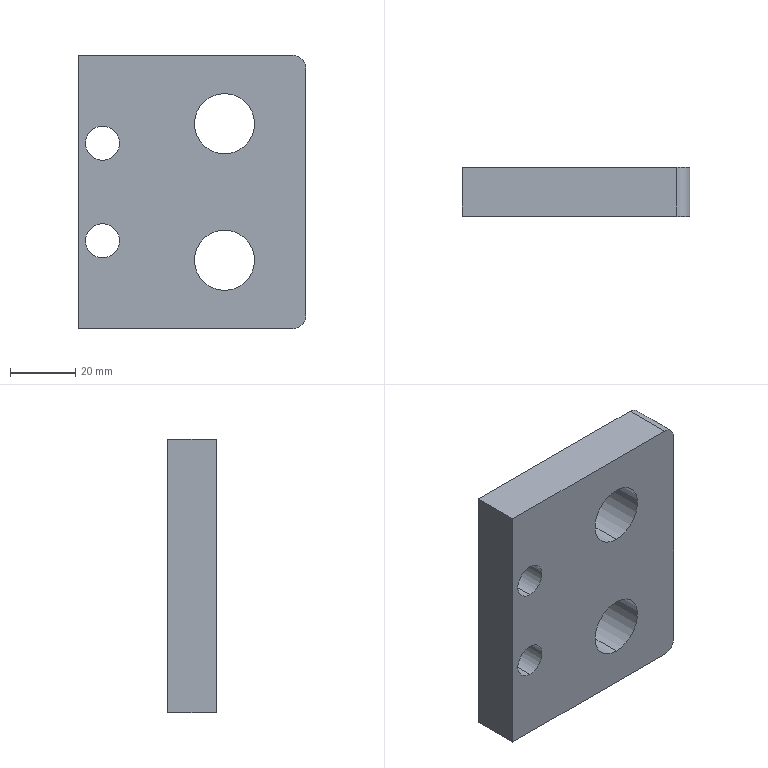Part | 1 solid | 16 faces | box 70 x 15 x 84 mm | volume 77435 mm3 | cylinder 10 | plane 6 | commonest cylinder face diameters 10.5 x4 18.5 x4 8 x2
STEP:
#1=CARTESIAN_POINT('',(10.,0.,-30.25));
#2=VERTEX_POINT('',#1);
#3=CARTESIAN_POINT('',(10.,0.,-11.75));
#4=VERTEX_POINT('',#3);
#5=CARTESIAN_POINT('',(10.,0.,-21.));
#6=DIRECTION('',(0.,1.,0.));
#7=DIRECTION('',(0.,0.,1.));
#8=AXIS2_PLACEMENT_3D('',#5,#6,#7);
#9=CIRCLE('',#8,9.25);
#10=EDGE_CURVE('',#2,#4,#9,.T.);
#11=ORIENTED_EDGE('',*,*,#10,.F.);
#12=CARTESIAN_POINT('',(10.,15.,-30.25));
#13=VERTEX_POINT('',#12);
#14=CARTESIAN_POINT('',(10.,15.,-30.25));
#15=DIRECTION('',(0.,1.,0.));
#16=VECTOR('',#15,1000.);
#17=LINE('',#14,#16);
#18=EDGE_CURVE('',#2,#13,#17,.T.);
#19=ORIENTED_EDGE('',*,*,#18,.T.);
#20=CARTESIAN_POINT('',(10.,15.,-11.75));
#21=VERTEX_POINT('',#20);
#22=CARTESIAN_POINT('',(10.,15.,-21.));
#23=DIRECTION('',(0.,1.,0.));
#24=DIRECTION('',(0.,0.,1.));
#25=AXIS2_PLACEMENT_3D('',#22,#23,#24);
#26=CIRCLE('',#25,9.25);
#27=EDGE_CURVE('',#13,#21,#26,.T.);
#28=ORIENTED_EDGE('',*,*,#27,.T.);
#29=CARTESIAN_POINT('',(10.,15.,-11.75));
#30=DIRECTION('',(0.,1.,0.));
#31=VECTOR('',#30,1000.);
#32=LINE('',#29,#31);
#33=EDGE_CURVE('',#4,#21,#32,.T.);
#34=ORIENTED_EDGE('',*,*,#33,.F.);
#35=EDGE_LOOP('',(#11,#19,#28,#34));
#36=FACE_OUTER_BOUND('',#35,.T.);
#37=CARTESIAN_POINT('',(10.,15.,-21.));
#38=DIRECTION('',(0.,1.,0.));
#39=DIRECTION('',(0.,0.,1.));
#40=AXIS2_PLACEMENT_3D('',#37,#38,#39);
#41=CYLINDRICAL_SURFACE('',#40,9.25);
#42=ADVANCED_FACE('',(#36),#41,.F.);
#43=CARTESIAN_POINT('',(10.,0.,11.75));
#44=VERTEX_POINT('',#43);
#45=CARTESIAN_POINT('',(10.,0.,30.25));
#46=VERTEX_POINT('',#45);
#47=CARTESIAN_POINT('',(10.,0.,21.));
#48=DIRECTION('',(0.,1.,0.));
#49=DIRECTION('',(0.,0.,1.));
#50=AXIS2_PLACEMENT_3D('',#47,#48,#49);
#51=CIRCLE('',#50,9.25);
#52=EDGE_CURVE('',#44,#46,#51,.T.);
#53=ORIENTED_EDGE('',*,*,#52,.F.);
#54=CARTESIAN_POINT('',(10.,15.,11.75));
#55=VERTEX_POINT('',#54);
#56=CARTESIAN_POINT('',(10.,15.,11.75));
#57=DIRECTION('',(0.,1.,0.));
#58=VECTOR('',#57,1000.);
#59=LINE('',#56,#58);
#60=EDGE_CURVE('',#44,#55,#59,.T.);
#61=ORIENTED_EDGE('',*,*,#60,.T.);
#62=CARTESIAN_POINT('',(10.,15.,30.25));
#63=VERTEX_POINT('',#62);
#64=CARTESIAN_POINT('',(10.,15.,21.));
#65=DIRECTION('',(0.,1.,0.));
#66=DIRECTION('',(0.,0.,1.));
#67=AXIS2_PLACEMENT_3D('',#64,#65,#66);
#68=CIRCLE('',#67,9.25);
#69=EDGE_CURVE('',#55,#63,#68,.T.);
#70=ORIENTED_EDGE('',*,*,#69,.T.);
#71=CARTESIAN_POINT('',(10.,15.,30.25));
#72=DIRECTION('',(0.,1.,0.));
#73=VECTOR('',#72,1000.);
#74=LINE('',#71,#73);
#75=EDGE_CURVE('',#46,#63,#74,.T.);
#76=ORIENTED_EDGE('',*,*,#75,.F.);
#77=EDGE_LOOP('',(#53,#61,#70,#76));
#78=FACE_OUTER_BOUND('',#77,.T.);
#79=CARTESIAN_POINT('',(10.,15.,21.));
#80=DIRECTION('',(0.,1.,0.));
#81=DIRECTION('',(0.,0.,1.));
#82=AXIS2_PLACEMENT_3D('',#79,#80,#81);
#83=CYLINDRICAL_SURFACE('',#82,9.25);
#84=ADVANCED_FACE('',(#78),#83,.F.);
#85=CARTESIAN_POINT('',(-27.5,15.,9.75));
#86=VERTEX_POINT('',#85);
#87=CARTESIAN_POINT('',(-27.5,15.,20.25));
#88=VERTEX_POINT('',#87);
#89=CARTESIAN_POINT('',(-27.5,15.,15.));
#90=DIRECTION('',(0.,1.,0.));
#91=DIRECTION('',(0.,0.,1.));
#92=AXIS2_PLACEMENT_3D('',#89,#90,#91);
#93=CIRCLE('',#92,5.25);
#94=EDGE_CURVE('',#86,#88,#93,.T.);
#95=ORIENTED_EDGE('',*,*,#94,.T.);
#96=CARTESIAN_POINT('',(-27.5,0.,20.25));
#97=VERTEX_POINT('',#96);
#98=CARTESIAN_POINT('',(-27.5,15.,20.25));
#99=DIRECTION('',(0.,-1.,0.));
#100=VECTOR('',#99,1000.);
#101=LINE('',#98,#100);
#102=EDGE_CURVE('',#88,#97,#101,.T.);
#103=ORIENTED_EDGE('',*,*,#102,.T.);
#104=CARTESIAN_POINT('',(-27.5,0.,9.75));
#105=VERTEX_POINT('',#104);
#106=CARTESIAN_POINT('',(-27.5,0.,15.));
#107=DIRECTION('',(0.,1.,0.));
#108=DIRECTION('',(0.,0.,1.));
#109=AXIS2_PLACEMENT_3D('',#106,#107,#108);
#110=CIRCLE('',#109,5.25);
#111=EDGE_CURVE('',#105,#97,#110,.T.);
#112=ORIENTED_EDGE('',*,*,#111,.F.);
#113=CARTESIAN_POINT('',(-27.5,15.,9.75));
#114=DIRECTION('',(0.,-1.,0.));
#115=VECTOR('',#114,1000.);
#116=LINE('',#113,#115);
#117=EDGE_CURVE('',#86,#105,#116,.T.);
#118=ORIENTED_EDGE('',*,*,#117,.F.);
#119=EDGE_LOOP('',(#95,#103,#112,#118));
#120=FACE_OUTER_BOUND('',#119,.T.);
#121=CARTESIAN_POINT('',(-27.5,15.,15.));
#122=DIRECTION('',(0.,-1.,0.));
#123=DIRECTION('',(0.,0.,-1.));
#124=AXIS2_PLACEMENT_3D('',#121,#122,#123);
#125=CYLINDRICAL_SURFACE('',#124,5.25);
#126=ADVANCED_FACE('',(#120),#125,.F.);
#127=CARTESIAN_POINT('',(-27.5,15.,-20.25));
#128=VERTEX_POINT('',#127);
#129=CARTESIAN_POINT('',(-27.5,15.,-9.75));
#130=VERTEX_POINT('',#129);
#131=CARTESIAN_POINT('',(-27.5,15.,-15.));
#132=DIRECTION('',(0.,1.,0.));
#133=DIRECTION('',(0.,0.,1.));
#134=AXIS2_PLACEMENT_3D('',#131,#132,#133);
#135=CIRCLE('',#134,5.25);
#136=EDGE_CURVE('',#128,#130,#135,.T.);
#137=ORIENTED_EDGE('',*,*,#136,.T.);
#138=CARTESIAN_POINT('',(-27.5,0.,-9.75));
#139=VERTEX_POINT('',#138);
#140=CARTESIAN_POINT('',(-27.5,15.,-9.75));
#141=DIRECTION('',(0.,-1.,0.));
#142=VECTOR('',#141,1000.);
#143=LINE('',#140,#142);
#144=EDGE_CURVE('',#130,#139,#143,.T.);
#145=ORIENTED_EDGE('',*,*,#144,.T.);
#146=CARTESIAN_POINT('',(-27.5,0.,-20.25));
#147=VERTEX_POINT('',#146);
#148=CARTESIAN_POINT('',(-27.5,0.,-15.));
#149=DIRECTION('',(0.,1.,0.));
#150=DIRECTION('',(0.,0.,1.));
#151=AXIS2_PLACEMENT_3D('',#148,#149,#150);
#152=CIRCLE('',#151,5.25);
#153=EDGE_CURVE('',#147,#139,#152,.T.);
#154=ORIENTED_EDGE('',*,*,#153,.F.);
#155=CARTESIAN_POINT('',(-27.5,15.,-20.25));
#156=DIRECTION('',(0.,-1.,0.));
#157=VECTOR('',#156,1000.);
#158=LINE('',#155,#157);
#159=EDGE_CURVE('',#128,#147,#158,.T.);
#160=ORIENTED_EDGE('',*,*,#159,.F.);
#161=EDGE_LOOP('',(#137,#145,#154,#160));
#162=FACE_OUTER_BOUND('',#161,.T.);
#163=CARTESIAN_POINT('',(-27.5,15.,-15.));
#164=DIRECTION('',(0.,-1.,0.));
#165=DIRECTION('',(0.,0.,-1.));
#166=AXIS2_PLACEMENT_3D('',#163,#164,#165);
#167=CYLINDRICAL_SURFACE('',#166,5.25);
#168=ADVANCED_FACE('',(#162),#167,.F.);
#169=CARTESIAN_POINT('',(10.,15.,-21.));
#170=DIRECTION('',(0.,1.,0.));
#171=DIRECTION('',(0.,0.,1.));
#172=AXIS2_PLACEMENT_3D('',#169,#170,#171);
#173=CIRCLE('',#172,9.25);
#174=EDGE_CURVE('',#21,#13,#173,.T.);
#175=ORIENTED_EDGE('',*,*,#174,.F.);
#176=ORIENTED_EDGE('',*,*,#27,.F.);
#177=EDGE_LOOP('',(#175,#176));
#178=FACE_BOUND('',#177,.T.);
#179=CARTESIAN_POINT('',(10.,15.,21.));
#180=DIRECTION('',(0.,1.,0.));
#181=DIRECTION('',(0.,0.,1.));
#182=AXIS2_PLACEMENT_3D('',#179,#180,#181);
#183=CIRCLE('',#182,9.25);
#184=EDGE_CURVE('',#63,#55,#183,.T.);
#185=ORIENTED_EDGE('',*,*,#184,.F.);
#186=ORIENTED_EDGE('',*,*,#69,.F.);
#187=EDGE_LOOP('',(#185,#186));
#188=FACE_BOUND('',#187,.T.);
#189=ORIENTED_EDGE('',*,*,#136,.F.);
#190=CARTESIAN_POINT('',(-27.5,15.,-15.));
#191=DIRECTION('',(0.,1.,0.));
#192=DIRECTION('',(0.,0.,1.));
#193=AXIS2_PLACEMENT_3D('',#190,#191,#192);
#194=CIRCLE('',#193,5.25);
#195=EDGE_CURVE('',#130,#128,#194,.T.);
#196=ORIENTED_EDGE('',*,*,#195,.F.);
#197=EDGE_LOOP('',(#189,#196));
#198=FACE_BOUND('',#197,.T.);
#199=CARTESIAN_POINT('',(-35.,15.,-42.));
#200=VERTEX_POINT('',#199);
#201=CARTESIAN_POINT('',(-35.,15.,42.));
#202=VERTEX_POINT('',#201);
#203=CARTESIAN_POINT('',(-35.,15.,-42.));
#204=DIRECTION('',(0.,0.,1.));
#205=VECTOR('',#204,1000.);
#206=LINE('',#203,#205);
#207=EDGE_CURVE('',#200,#202,#206,.T.);
#208=ORIENTED_EDGE('',*,*,#207,.T.);
#209=CARTESIAN_POINT('',(31.,15.,42.));
#210=VERTEX_POINT('',#209);
#211=CARTESIAN_POINT('',(-35.,15.,42.));
#212=DIRECTION('',(1.,0.,0.));
#213=VECTOR('',#212,1000.);
#214=LINE('',#211,#213);
#215=EDGE_CURVE('',#202,#210,#214,.T.);
#216=ORIENTED_EDGE('',*,*,#215,.T.);
#217=CARTESIAN_POINT('',(35.,15.,38.));
#218=VERTEX_POINT('',#217);
#219=CARTESIAN_POINT('',(31.,15.,38.));
#220=DIRECTION('',(0.,1.,0.));
#221=DIRECTION('',(0.,0.,1.));
#222=AXIS2_PLACEMENT_3D('',#219,#220,#221);
#223=CIRCLE('',#222,4.);
#224=EDGE_CURVE('',#210,#218,#223,.T.);
#225=ORIENTED_EDGE('',*,*,#224,.T.);
#226=CARTESIAN_POINT('',(35.,15.,-38.));
#227=VERTEX_POINT('',#226);
#228=CARTESIAN_POINT('',(35.,15.,-38.));
#229=DIRECTION('',(0.,0.,-1.));
#230=VECTOR('',#229,1000.);
#231=LINE('',#228,#230);
#232=EDGE_CURVE('',#218,#227,#231,.T.);
#233=ORIENTED_EDGE('',*,*,#232,.T.);
#234=CARTESIAN_POINT('',(31.,15.,-42.));
#235=VERTEX_POINT('',#234);
#236=CARTESIAN_POINT('',(31.,15.,-38.));
#237=DIRECTION('',(0.,1.,0.));
#238=DIRECTION('',(0.,0.,-1.));
#239=AXIS2_PLACEMENT_3D('',#236,#237,#238);
#240=CIRCLE('',#239,4.);
#241=EDGE_CURVE('',#227,#235,#240,.T.);
#242=ORIENTED_EDGE('',*,*,#241,.T.);
#243=CARTESIAN_POINT('',(-35.,15.,-42.));
#244=DIRECTION('',(-1.,0.,0.));
#245=VECTOR('',#244,1000.);
#246=LINE('',#243,#245);
#247=EDGE_CURVE('',#235,#200,#246,.T.);
#248=ORIENTED_EDGE('',*,*,#247,.T.);
#249=EDGE_LOOP('',(#208,#216,#225,#233,#242,#248));
#250=FACE_OUTER_BOUND('',#249,.T.);
#251=ORIENTED_EDGE('',*,*,#94,.F.);
#252=CARTESIAN_POINT('',(-27.5,15.,15.));
#253=DIRECTION('',(0.,1.,0.));
#254=DIRECTION('',(0.,0.,1.));
#255=AXIS2_PLACEMENT_3D('',#252,#253,#254);
#256=CIRCLE('',#255,5.25);
#257=EDGE_CURVE('',#88,#86,#256,.T.);
#258=ORIENTED_EDGE('',*,*,#257,.F.);
#259=EDGE_LOOP('',(#251,#258));
#260=FACE_BOUND('',#259,.T.);
#261=CARTESIAN_POINT('',(31.,15.,38.));
#262=DIRECTION('',(0.,1.,0.));
#263=DIRECTION('',(0.,0.,1.));
#264=AXIS2_PLACEMENT_3D('',#261,#262,#263);
#265=PLANE('',#264);
#266=ADVANCED_FACE('',(#178,#188,#198,#250,#260),#265,.T.);
#267=CARTESIAN_POINT('',(10.,0.,-21.));
#268=DIRECTION('',(0.,1.,0.));
#269=DIRECTION('',(0.,0.,1.));
#270=AXIS2_PLACEMENT_3D('',#267,#268,#269);
#271=CIRCLE('',#270,9.25);
#272=EDGE_CURVE('',#4,#2,#271,.T.);
#273=ORIENTED_EDGE('',*,*,#272,.T.);
#274=ORIENTED_EDGE('',*,*,#10,.T.);
#275=EDGE_LOOP('',(#273,#274));
#276=FACE_BOUND('',#275,.T.);
#277=CARTESIAN_POINT('',(10.,0.,21.));
#278=DIRECTION('',(0.,1.,0.));
#279=DIRECTION('',(0.,0.,1.));
#280=AXIS2_PLACEMENT_3D('',#277,#278,#279);
#281=CIRCLE('',#280,9.25);
#282=EDGE_CURVE('',#46,#44,#281,.T.);
#283=ORIENTED_EDGE('',*,*,#282,.T.);
#284=ORIENTED_EDGE('',*,*,#52,.T.);
#285=EDGE_LOOP('',(#283,#284));
#286=FACE_BOUND('',#285,.T.);
#287=CARTESIAN_POINT('',(-35.,0.,-42.));
#288=VERTEX_POINT('',#287);
#289=CARTESIAN_POINT('',(-35.,0.,42.));
#290=VERTEX_POINT('',#289);
#291=CARTESIAN_POINT('',(-35.,0.,-42.));
#292=DIRECTION('',(0.,0.,1.));
#293=VECTOR('',#292,1000.);
#294=LINE('',#291,#293);
#295=EDGE_CURVE('',#288,#290,#294,.T.);
#296=ORIENTED_EDGE('',*,*,#295,.F.);
#297=CARTESIAN_POINT('',(31.,0.,-42.));
#298=VERTEX_POINT('',#297);
#299=CARTESIAN_POINT('',(-35.,0.,-42.));
#300=DIRECTION('',(-1.,0.,0.));
#301=VECTOR('',#300,1000.);
#302=LINE('',#299,#301);
#303=EDGE_CURVE('',#298,#288,#302,.T.);
#304=ORIENTED_EDGE('',*,*,#303,.F.);
#305=CARTESIAN_POINT('',(35.,0.,-38.));
#306=VERTEX_POINT('',#305);
#307=CARTESIAN_POINT('',(31.,0.,-38.));
#308=DIRECTION('',(0.,1.,0.));
#309=DIRECTION('',(0.,0.,-1.));
#310=AXIS2_PLACEMENT_3D('',#307,#308,#309);
#311=CIRCLE('',#310,4.);
#312=EDGE_CURVE('',#306,#298,#311,.T.);
#313=ORIENTED_EDGE('',*,*,#312,.F.);
#314=CARTESIAN_POINT('',(35.,0.,38.));
#315=VERTEX_POINT('',#314);
#316=CARTESIAN_POINT('',(35.,0.,-38.));
#317=DIRECTION('',(0.,0.,-1.));
#318=VECTOR('',#317,1000.);
#319=LINE('',#316,#318);
#320=EDGE_CURVE('',#315,#306,#319,.T.);
#321=ORIENTED_EDGE('',*,*,#320,.F.);
#322=CARTESIAN_POINT('',(31.,0.,42.));
#323=VERTEX_POINT('',#322);
#324=CARTESIAN_POINT('',(31.,0.,38.));
#325=DIRECTION('',(0.,1.,0.));
#326=DIRECTION('',(0.,0.,1.));
#327=AXIS2_PLACEMENT_3D('',#324,#325,#326);
#328=CIRCLE('',#327,4.);
#329=EDGE_CURVE('',#323,#315,#328,.T.);
#330=ORIENTED_EDGE('',*,*,#329,.F.);
#331=CARTESIAN_POINT('',(-35.,0.,42.));
#332=DIRECTION('',(1.,0.,0.));
#333=VECTOR('',#332,1000.);
#334=LINE('',#331,#333);
#335=EDGE_CURVE('',#290,#323,#334,.T.);
#336=ORIENTED_EDGE('',*,*,#335,.F.);
#337=EDGE_LOOP('',(#296,#304,#313,#321,#330,#336));
#338=FACE_OUTER_BOUND('',#337,.T.);
#339=ORIENTED_EDGE('',*,*,#153,.T.);
#340=CARTESIAN_POINT('',(-27.5,0.,-15.));
#341=DIRECTION('',(0.,1.,0.));
#342=DIRECTION('',(0.,0.,1.));
#343=AXIS2_PLACEMENT_3D('',#340,#341,#342);
#344=CIRCLE('',#343,5.25);
#345=EDGE_CURVE('',#139,#147,#344,.T.);
#346=ORIENTED_EDGE('',*,*,#345,.T.);
#347=EDGE_LOOP('',(#339,#346));
#348=FACE_BOUND('',#347,.T.);
#349=ORIENTED_EDGE('',*,*,#111,.T.);
#350=CARTESIAN_POINT('',(-27.5,0.,15.));
#351=DIRECTION('',(0.,1.,0.));
#352=DIRECTION('',(0.,0.,1.));
#353=AXIS2_PLACEMENT_3D('',#350,#351,#352);
#354=CIRCLE('',#353,5.25);
#355=EDGE_CURVE('',#97,#105,#354,.T.);
#356=ORIENTED_EDGE('',*,*,#355,.T.);
#357=EDGE_LOOP('',(#349,#356));
#358=FACE_BOUND('',#357,.T.);
#359=CARTESIAN_POINT('',(31.,0.,38.));
#360=DIRECTION('',(0.,1.,0.));
#361=DIRECTION('',(0.,0.,1.));
#362=AXIS2_PLACEMENT_3D('',#359,#360,#361);
#363=PLANE('',#362);
#364=ADVANCED_FACE('',(#276,#286,#338,#348,#358),#363,.F.);
#365=ORIENTED_EDGE('',*,*,#295,.T.);
#366=CARTESIAN_POINT('',(-35.,15.,42.));
#367=DIRECTION('',(0.,-1.,0.));
#368=VECTOR('',#367,1000.);
#369=LINE('',#366,#368);
#370=EDGE_CURVE('',#202,#290,#369,.T.);
#371=ORIENTED_EDGE('',*,*,#370,.F.);
#372=ORIENTED_EDGE('',*,*,#207,.F.);
#373=CARTESIAN_POINT('',(-35.,15.,-42.));
#374=DIRECTION('',(0.,-1.,0.));
#375=VECTOR('',#374,1000.);
#376=LINE('',#373,#375);
#377=EDGE_CURVE('',#200,#288,#376,.T.);
#378=ORIENTED_EDGE('',*,*,#377,.T.);
#379=EDGE_LOOP('',(#365,#371,#372,#378));
#380=FACE_OUTER_BOUND('',#379,.T.);
#381=CARTESIAN_POINT('',(-35.,15.,-42.));
#382=DIRECTION('',(1.,0.,0.));
#383=DIRECTION('',(0.,0.,-1.));
#384=AXIS2_PLACEMENT_3D('',#381,#382,#383);
#385=PLANE('',#384);
#386=ADVANCED_FACE('',(#380),#385,.F.);
#387=ORIENTED_EDGE('',*,*,#335,.T.);
#388=CARTESIAN_POINT('',(31.,15.,42.));
#389=DIRECTION('',(0.,-1.,0.));
#390=VECTOR('',#389,1000.);
#391=LINE('',#388,#390);
#392=EDGE_CURVE('',#210,#323,#391,.T.);
#393=ORIENTED_EDGE('',*,*,#392,.F.);
#394=ORIENTED_EDGE('',*,*,#215,.F.);
#395=ORIENTED_EDGE('',*,*,#370,.T.);
#396=EDGE_LOOP('',(#387,#393,#394,#395));
#397=FACE_OUTER_BOUND('',#396,.T.);
#398=CARTESIAN_POINT('',(-35.,15.,42.));
#399=DIRECTION('',(0.,0.,-1.));
#400=DIRECTION('',(-1.,0.,0.));
#401=AXIS2_PLACEMENT_3D('',#398,#399,#400);
#402=PLANE('',#401);
#403=ADVANCED_FACE('',(#397),#402,.F.);
#404=ORIENTED_EDGE('',*,*,#329,.T.);
#405=CARTESIAN_POINT('',(35.,15.,38.));
#406=DIRECTION('',(0.,-1.,0.));
#407=VECTOR('',#406,1000.);
#408=LINE('',#405,#407);
#409=EDGE_CURVE('',#218,#315,#408,.T.);
#410=ORIENTED_EDGE('',*,*,#409,.F.);
#411=ORIENTED_EDGE('',*,*,#224,.F.);
#412=ORIENTED_EDGE('',*,*,#392,.T.);
#413=EDGE_LOOP('',(#404,#410,#411,#412));
#414=FACE_OUTER_BOUND('',#413,.T.);
#415=CARTESIAN_POINT('',(31.,15.,38.));
#416=DIRECTION('',(0.,-1.,0.));
#417=DIRECTION('',(0.,0.,-1.));
#418=AXIS2_PLACEMENT_3D('',#415,#416,#417);
#419=CYLINDRICAL_SURFACE('',#418,4.);
#420=ADVANCED_FACE('',(#414),#419,.T.);
#421=ORIENTED_EDGE('',*,*,#320,.T.);
#422=CARTESIAN_POINT('',(35.,15.,-38.));
#423=DIRECTION('',(0.,-1.,0.));
#424=VECTOR('',#423,1000.);
#425=LINE('',#422,#424);
#426=EDGE_CURVE('',#227,#306,#425,.T.);
#427=ORIENTED_EDGE('',*,*,#426,.F.);
#428=ORIENTED_EDGE('',*,*,#232,.F.);
#429=ORIENTED_EDGE('',*,*,#409,.T.);
#430=EDGE_LOOP('',(#421,#427,#428,#429));
#431=FACE_OUTER_BOUND('',#430,.T.);
#432=CARTESIAN_POINT('',(35.,15.,-38.));
#433=DIRECTION('',(-1.,0.,0.));
#434=DIRECTION('',(0.,0.,1.));
#435=AXIS2_PLACEMENT_3D('',#432,#433,#434);
#436=PLANE('',#435);
#437=ADVANCED_FACE('',(#431),#436,.F.);
#438=ORIENTED_EDGE('',*,*,#312,.T.);
#439=CARTESIAN_POINT('',(31.,15.,-42.));
#440=DIRECTION('',(0.,-1.,0.));
#441=VECTOR('',#440,1000.);
#442=LINE('',#439,#441);
#443=EDGE_CURVE('',#235,#298,#442,.T.);
#444=ORIENTED_EDGE('',*,*,#443,.F.);
#445=ORIENTED_EDGE('',*,*,#241,.F.);
#446=ORIENTED_EDGE('',*,*,#426,.T.);
#447=EDGE_LOOP('',(#438,#444,#445,#446));
#448=FACE_OUTER_BOUND('',#447,.T.);
#449=CARTESIAN_POINT('',(31.,15.,-38.));
#450=DIRECTION('',(0.,-1.,0.));
#451=DIRECTION('',(0.,0.,-1.));
#452=AXIS2_PLACEMENT_3D('',#449,#450,#451);
#453=CYLINDRICAL_SURFACE('',#452,4.);
#454=ADVANCED_FACE('',(#448),#453,.T.);
#455=ORIENTED_EDGE('',*,*,#303,.T.);
#456=ORIENTED_EDGE('',*,*,#377,.F.);
#457=ORIENTED_EDGE('',*,*,#247,.F.);
#458=ORIENTED_EDGE('',*,*,#443,.T.);
#459=EDGE_LOOP('',(#455,#456,#457,#458));
#460=FACE_OUTER_BOUND('',#459,.T.);
#461=CARTESIAN_POINT('',(-35.,15.,-42.));
#462=DIRECTION('',(0.,0.,1.));
#463=DIRECTION('',(1.,0.,0.));
#464=AXIS2_PLACEMENT_3D('',#461,#462,#463);
#465=PLANE('',#464);
#466=ADVANCED_FACE('',(#460),#465,.F.);
#467=ORIENTED_EDGE('',*,*,#144,.F.);
#468=ORIENTED_EDGE('',*,*,#195,.T.);
#469=ORIENTED_EDGE('',*,*,#159,.T.);
#470=ORIENTED_EDGE('',*,*,#345,.F.);
#471=EDGE_LOOP('',(#467,#468,#469,#470));
#472=FACE_OUTER_BOUND('',#471,.T.);
#473=CARTESIAN_POINT('',(-27.5,15.,-15.));
#474=DIRECTION('',(0.,-1.,0.));
#475=DIRECTION('',(0.,0.,-1.));
#476=AXIS2_PLACEMENT_3D('',#473,#474,#475);
#477=CYLINDRICAL_SURFACE('',#476,5.25);
#478=ADVANCED_FACE('',(#472),#477,.F.);
#479=ORIENTED_EDGE('',*,*,#102,.F.);
#480=ORIENTED_EDGE('',*,*,#257,.T.);
#481=ORIENTED_EDGE('',*,*,#117,.T.);
#482=ORIENTED_EDGE('',*,*,#355,.F.);
#483=EDGE_LOOP('',(#479,#480,#481,#482));
#484=FACE_OUTER_BOUND('',#483,.T.);
#485=CARTESIAN_POINT('',(-27.5,15.,15.));
#486=DIRECTION('',(0.,-1.,0.));
#487=DIRECTION('',(0.,0.,-1.));
#488=AXIS2_PLACEMENT_3D('',#485,#486,#487);
#489=CYLINDRICAL_SURFACE('',#488,5.25);
#490=ADVANCED_FACE('',(#484),#489,.F.);
#491=ORIENTED_EDGE('',*,*,#60,.F.);
#492=ORIENTED_EDGE('',*,*,#282,.F.);
#493=ORIENTED_EDGE('',*,*,#75,.T.);
#494=ORIENTED_EDGE('',*,*,#184,.T.);
#495=EDGE_LOOP('',(#491,#492,#493,#494));
#496=FACE_OUTER_BOUND('',#495,.T.);
#497=CARTESIAN_POINT('',(10.,15.,21.));
#498=DIRECTION('',(0.,1.,0.));
#499=DIRECTION('',(0.,0.,1.));
#500=AXIS2_PLACEMENT_3D('',#497,#498,#499);
#501=CYLINDRICAL_SURFACE('',#500,9.25);
#502=ADVANCED_FACE('',(#496),#501,.F.);
#503=ORIENTED_EDGE('',*,*,#18,.F.);
#504=ORIENTED_EDGE('',*,*,#272,.F.);
#505=ORIENTED_EDGE('',*,*,#33,.T.);
#506=ORIENTED_EDGE('',*,*,#174,.T.);
#507=EDGE_LOOP('',(#503,#504,#505,#506));
#508=FACE_OUTER_BOUND('',#507,.T.);
#509=CARTESIAN_POINT('',(10.,15.,-21.));
#510=DIRECTION('',(0.,1.,0.));
#511=DIRECTION('',(0.,0.,1.));
#512=AXIS2_PLACEMENT_3D('',#509,#510,#511);
#513=CYLINDRICAL_SURFACE('',#512,9.25);
#514=ADVANCED_FACE('',(#508),#513,.F.);
#515=CLOSED_SHELL('',(#42,#84,#126,#168,#266,#364,#386,#403,#420,#437,#454,#466,#478,#490,#502,#514));
#516=MANIFOLD_SOLID_BREP('',#515);
#517=CARTESIAN_POINT('',(0.,0.,0.));
#518=DIRECTION('',(0.,0.,1.));
#519=DIRECTION('',(1.,0.,0.));
#520=AXIS2_PLACEMENT_3D('',#517,#518,#519);
#521=(LENGTH_UNIT()NAMED_UNIT(*)SI_UNIT(.MILLI.,.METRE.));
#522=UNCERTAINTY_MEASURE_WITH_UNIT(LENGTH_MEASURE(0.00001),#521,'','');
#523=(NAMED_UNIT(*)PLANE_ANGLE_UNIT()SI_UNIT($,.RADIAN.));
#524=(NAMED_UNIT(*)SI_UNIT($,.STERADIAN.)SOLID_ANGLE_UNIT());
#525=(GEOMETRIC_REPRESENTATION_CONTEXT(3)GLOBAL_UNCERTAINTY_ASSIGNED_CONTEXT((#522))GLOBAL_UNIT_ASSIGNED_CONTEXT((#521,#523,#524))REPRESENTATION_CONTEXT('',''));
#526=ADVANCED_BREP_SHAPE_REPRESENTATION('',(#516,#520),#525);